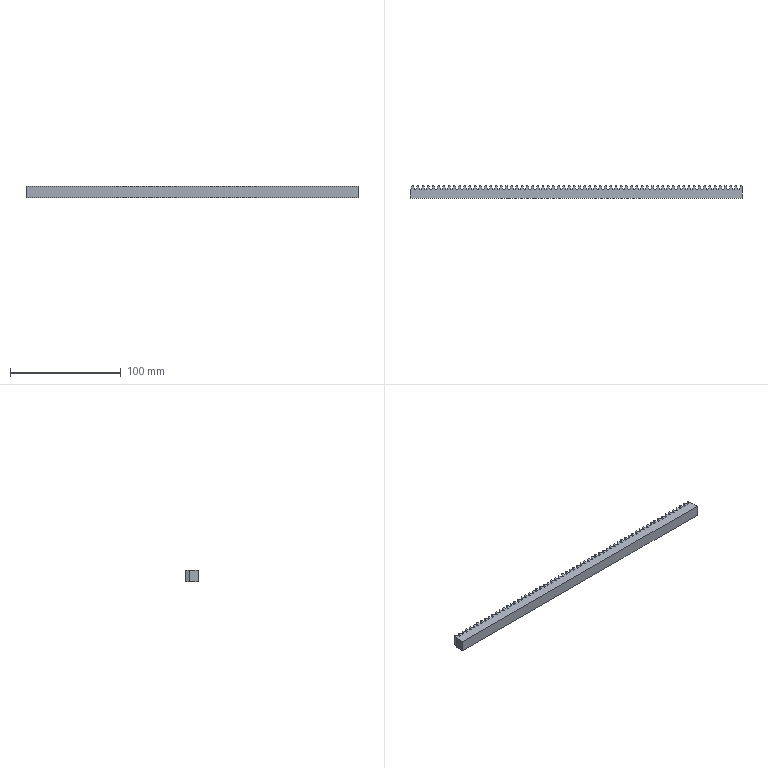Part | STEP file | rack spur rectangular_gb_GB - Rack-spur - rectangular 1.5M 20PA 10FW 10PH 300L---SAll | 1 solid | 261 faces | box 300 x 11.5 x 10 mm | volume 29060 mm3 | plane 261